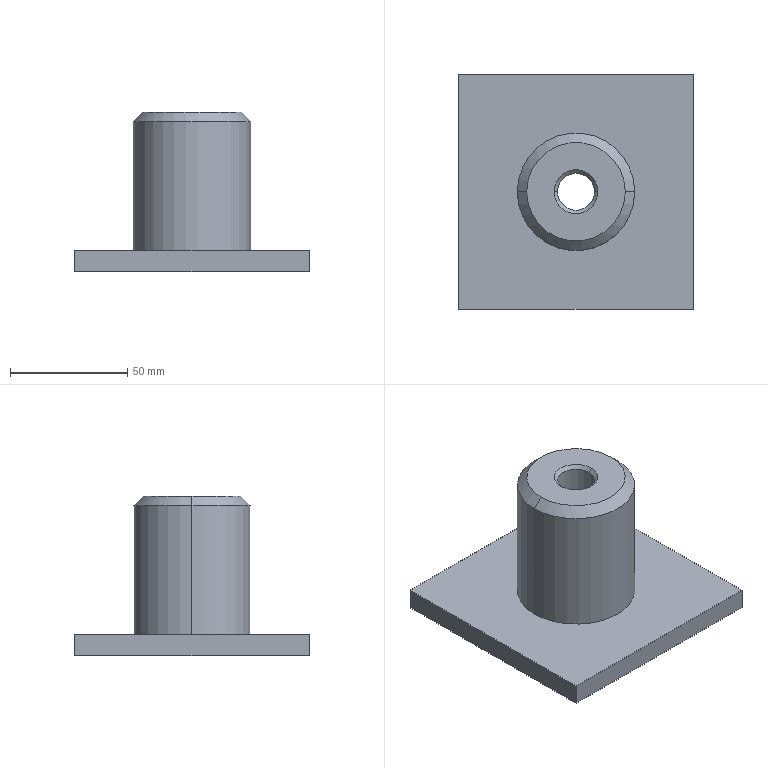Part | SolidWorks | features Chamfer 1, Extrusion 1, HoleWzd 1, ICE 1 | 1 solid | 17 faces | box 100 x 100 x 68 mm | volume 174571 mm3 | plane 7 | cone 6 | cylinder 4 | commonest cylinder face diameters 24 x2 50 x2
STEP:
#1=CARTESIAN_POINT('',(21.,0.,68.));
#2=VERTEX_POINT('',#1);
#3=CARTESIAN_POINT('',(-21.,0.,68.));
#4=VERTEX_POINT('',#3);
#5=CARTESIAN_POINT('',(0.,0.,68.));
#6=DIRECTION('',(0.,0.,1.));
#7=DIRECTION('',(1.,0.,0.));
#8=AXIS2_PLACEMENT_3D('',#5,#6,#7);
#9=CIRCLE('',#8,21.);
#10=EDGE_CURVE('',#2,#4,#9,.T.);
#11=ORIENTED_EDGE('',*,*,#10,.F.);
#12=CARTESIAN_POINT('',(25.,0.,64.));
#13=VERTEX_POINT('',#12);
#14=CARTESIAN_POINT('',(21.,0.,68.));
#15=DIRECTION('',(0.7071,0.,-0.7071));
#16=VECTOR('',#15,1000.);
#17=LINE('',#14,#16);
#18=EDGE_CURVE('',#2,#13,#17,.T.);
#19=ORIENTED_EDGE('',*,*,#18,.T.);
#20=CARTESIAN_POINT('',(-25.,0.,64.));
#21=VERTEX_POINT('',#20);
#22=CARTESIAN_POINT('',(0.,0.,64.));
#23=DIRECTION('',(0.,0.,-1.));
#24=DIRECTION('',(1.,0.,0.));
#25=AXIS2_PLACEMENT_3D('',#22,#23,#24);
#26=CIRCLE('',#25,25.);
#27=EDGE_CURVE('',#21,#13,#26,.T.);
#28=ORIENTED_EDGE('',*,*,#27,.F.);
#29=CARTESIAN_POINT('',(-21.,0.,68.));
#30=DIRECTION('',(-0.7071,0.,-0.7071));
#31=VECTOR('',#30,1000.);
#32=LINE('',#29,#31);
#33=EDGE_CURVE('',#4,#21,#32,.T.);
#34=ORIENTED_EDGE('',*,*,#33,.F.);
#35=EDGE_LOOP('',(#11,#19,#28,#34));
#36=FACE_OUTER_BOUND('',#35,.T.);
#37=CARTESIAN_POINT('',(0.,0.,68.));
#38=DIRECTION('',(0.,0.,-1.));
#39=DIRECTION('',(-1.,0.,0.));
#40=AXIS2_PLACEMENT_3D('',#37,#38,#39);
#41=CONICAL_SURFACE('',#40,21.,0.7854);
#42=ADVANCED_FACE('',(#36),#41,.T.);
#43=CARTESIAN_POINT('',(-7.842,0.,66.499));
#44=VERTEX_POINT('',#43);
#45=CARTESIAN_POINT('',(7.842,0.,66.499));
#46=VERTEX_POINT('',#45);
#47=CARTESIAN_POINT('',(0.,0.,66.499));
#48=DIRECTION('',(0.,0.,1.));
#49=DIRECTION('',(-1.,0.,0.));
#50=AXIS2_PLACEMENT_3D('',#47,#48,#49);
#51=CIRCLE('',#50,7.842);
#52=EDGE_CURVE('',#44,#46,#51,.T.);
#53=ORIENTED_EDGE('',*,*,#52,.F.);
#54=CARTESIAN_POINT('',(-9.343,0.,68.));
#55=VERTEX_POINT('',#54);
#56=CARTESIAN_POINT('',(-7.842,0.,66.499));
#57=DIRECTION('',(-0.7071,0.,0.7071));
#58=VECTOR('',#57,1000.);
#59=LINE('',#56,#58);
#60=EDGE_CURVE('',#44,#55,#59,.T.);
#61=ORIENTED_EDGE('',*,*,#60,.T.);
#62=CARTESIAN_POINT('',(9.343,0.,68.));
#63=VERTEX_POINT('',#62);
#64=CARTESIAN_POINT('',(0.,0.,68.));
#65=DIRECTION('',(0.,0.,-1.));
#66=DIRECTION('',(1.,0.,0.));
#67=AXIS2_PLACEMENT_3D('',#64,#65,#66);
#68=CIRCLE('',#67,9.343);
#69=EDGE_CURVE('',#63,#55,#68,.T.);
#70=ORIENTED_EDGE('',*,*,#69,.F.);
#71=CARTESIAN_POINT('',(7.842,0.,66.499));
#72=DIRECTION('',(0.7071,0.,0.7071));
#73=VECTOR('',#72,1000.);
#74=LINE('',#71,#73);
#75=EDGE_CURVE('',#46,#63,#74,.T.);
#76=ORIENTED_EDGE('',*,*,#75,.F.);
#77=EDGE_LOOP('',(#53,#61,#70,#76));
#78=FACE_OUTER_BOUND('',#77,.T.);
#79=CARTESIAN_POINT('',(0.,0.,66.499));
#80=DIRECTION('',(0.,0.,1.));
#81=DIRECTION('',(1.,0.,0.));
#82=AXIS2_PLACEMENT_3D('',#79,#80,#81);
#83=CONICAL_SURFACE('',#82,7.842,0.7854);
#84=ADVANCED_FACE('',(#78),#83,.F.);
#85=CARTESIAN_POINT('',(12.,0.,64.));
#86=VERTEX_POINT('',#85);
#87=CARTESIAN_POINT('',(-12.,0.,64.));
#88=VERTEX_POINT('',#87);
#89=CARTESIAN_POINT('',(0.,0.,64.));
#90=DIRECTION('',(0.,0.,-1.));
#91=DIRECTION('',(-1.,0.,0.));
#92=AXIS2_PLACEMENT_3D('',#89,#90,#91);
#93=CIRCLE('',#92,12.);
#94=EDGE_CURVE('',#86,#88,#93,.T.);
#95=ORIENTED_EDGE('',*,*,#94,.F.);
#96=CARTESIAN_POINT('',(12.,0.,0.));
#97=VERTEX_POINT('',#96);
#98=CARTESIAN_POINT('',(12.,0.,0.));
#99=DIRECTION('',(0.,0.,-1.));
#100=VECTOR('',#99,1000.);
#101=LINE('',#98,#100);
#102=EDGE_CURVE('',#86,#97,#101,.T.);
#103=ORIENTED_EDGE('',*,*,#102,.T.);
#104=CARTESIAN_POINT('',(-12.,0.,0.));
#105=VERTEX_POINT('',#104);
#106=CARTESIAN_POINT('',(0.,0.,0.));
#107=DIRECTION('',(0.,0.,-1.));
#108=DIRECTION('',(-1.,0.,0.));
#109=AXIS2_PLACEMENT_3D('',#106,#107,#108);
#110=CIRCLE('',#109,12.);
#111=EDGE_CURVE('',#97,#105,#110,.T.);
#112=ORIENTED_EDGE('',*,*,#111,.T.);
#113=CARTESIAN_POINT('',(-12.,0.,0.));
#114=DIRECTION('',(0.,0.,-1.));
#115=VECTOR('',#114,1000.);
#116=LINE('',#113,#115);
#117=EDGE_CURVE('',#88,#105,#116,.T.);
#118=ORIENTED_EDGE('',*,*,#117,.F.);
#119=EDGE_LOOP('',(#95,#103,#112,#118));
#120=FACE_OUTER_BOUND('',#119,.T.);
#121=CARTESIAN_POINT('',(0.,0.,0.));
#122=DIRECTION('',(0.,0.,-1.));
#123=DIRECTION('',(-1.,0.,0.));
#124=AXIS2_PLACEMENT_3D('',#121,#122,#123);
#125=CYLINDRICAL_SURFACE('',#124,12.);
#126=ADVANCED_FACE('',(#120),#125,.F.);
#127=ORIENTED_EDGE('',*,*,#52,.T.);
#128=CARTESIAN_POINT('',(12.,0.,64.));
#129=DIRECTION('',(0.8572,0.,-0.515));
#130=VECTOR('',#129,1000.);
#131=LINE('',#128,#130);
#132=EDGE_CURVE('',#46,#86,#131,.T.);
#133=ORIENTED_EDGE('',*,*,#132,.T.);
#134=ORIENTED_EDGE('',*,*,#94,.T.);
#135=CARTESIAN_POINT('',(-12.,0.,64.));
#136=DIRECTION('',(-0.8572,0.,-0.515));
#137=VECTOR('',#136,1000.);
#138=LINE('',#135,#137);
#139=EDGE_CURVE('',#44,#88,#138,.T.);
#140=ORIENTED_EDGE('',*,*,#139,.F.);
#141=EDGE_LOOP('',(#127,#133,#134,#140));
#142=FACE_OUTER_BOUND('',#141,.T.);
#143=CARTESIAN_POINT('',(0.,0.,64.));
#144=DIRECTION('',(0.,0.,-1.));
#145=DIRECTION('',(-1.,0.,0.));
#146=AXIS2_PLACEMENT_3D('',#143,#144,#145);
#147=CONICAL_SURFACE('',#146,12.,1.03);
#148=ADVANCED_FACE('',(#142),#147,.F.);
#149=ORIENTED_EDGE('',*,*,#27,.T.);
#150=CARTESIAN_POINT('',(25.,0.,9.));
#151=VERTEX_POINT('',#150);
#152=CARTESIAN_POINT('',(25.,0.,68.));
#153=DIRECTION('',(0.,0.,-1.));
#154=VECTOR('',#153,1000.);
#155=LINE('',#152,#154);
#156=EDGE_CURVE('',#13,#151,#155,.T.);
#157=ORIENTED_EDGE('',*,*,#156,.T.);
#158=CARTESIAN_POINT('',(-25.,0.,9.));
#159=VERTEX_POINT('',#158);
#160=CARTESIAN_POINT('',(0.,0.,9.));
#161=DIRECTION('',(0.,0.,1.));
#162=DIRECTION('',(1.,0.,0.));
#163=AXIS2_PLACEMENT_3D('',#160,#161,#162);
#164=CIRCLE('',#163,25.);
#165=EDGE_CURVE('',#151,#159,#164,.T.);
#166=ORIENTED_EDGE('',*,*,#165,.T.);
#167=CARTESIAN_POINT('',(-25.,0.,68.));
#168=DIRECTION('',(0.,0.,-1.));
#169=VECTOR('',#168,1000.);
#170=LINE('',#167,#169);
#171=EDGE_CURVE('',#21,#159,#170,.T.);
#172=ORIENTED_EDGE('',*,*,#171,.F.);
#173=EDGE_LOOP('',(#149,#157,#166,#172));
#174=FACE_OUTER_BOUND('',#173,.T.);
#175=CARTESIAN_POINT('',(0.,0.,68.));
#176=DIRECTION('',(0.,0.,-1.));
#177=DIRECTION('',(-1.,0.,0.));
#178=AXIS2_PLACEMENT_3D('',#175,#176,#177);
#179=CYLINDRICAL_SURFACE('',#178,25.);
#180=ADVANCED_FACE('',(#174),#179,.T.);
#181=CARTESIAN_POINT('',(-50.,50.,0.));
#182=VERTEX_POINT('',#181);
#183=CARTESIAN_POINT('',(-50.,-50.,0.));
#184=VERTEX_POINT('',#183);
#185=CARTESIAN_POINT('',(-50.,50.,0.));
#186=DIRECTION('',(0.,-1.,0.));
#187=VECTOR('',#186,1000.);
#188=LINE('',#185,#187);
#189=EDGE_CURVE('',#182,#184,#188,.T.);
#190=ORIENTED_EDGE('',*,*,#189,.T.);
#191=CARTESIAN_POINT('',(-50.,-50.,9.));
#192=VERTEX_POINT('',#191);
#193=CARTESIAN_POINT('',(-50.,-50.,9.));
#194=DIRECTION('',(0.,0.,-1.));
#195=VECTOR('',#194,1000.);
#196=LINE('',#193,#195);
#197=EDGE_CURVE('',#192,#184,#196,.T.);
#198=ORIENTED_EDGE('',*,*,#197,.F.);
#199=CARTESIAN_POINT('',(-50.,50.,9.));
#200=VERTEX_POINT('',#199);
#201=CARTESIAN_POINT('',(-50.,50.,9.));
#202=DIRECTION('',(0.,-1.,0.));
#203=VECTOR('',#202,1000.);
#204=LINE('',#201,#203);
#205=EDGE_CURVE('',#200,#192,#204,.T.);
#206=ORIENTED_EDGE('',*,*,#205,.F.);
#207=CARTESIAN_POINT('',(-50.,50.,9.));
#208=DIRECTION('',(0.,0.,-1.));
#209=VECTOR('',#208,1000.);
#210=LINE('',#207,#209);
#211=EDGE_CURVE('',#200,#182,#210,.T.);
#212=ORIENTED_EDGE('',*,*,#211,.T.);
#213=EDGE_LOOP('',(#190,#198,#206,#212));
#214=FACE_OUTER_BOUND('',#213,.T.);
#215=CARTESIAN_POINT('',(-50.,50.,9.));
#216=DIRECTION('',(1.,0.,0.));
#217=DIRECTION('',(0.,1.,0.));
#218=AXIS2_PLACEMENT_3D('',#215,#216,#217);
#219=PLANE('',#218);
#220=ADVANCED_FACE('',(#214),#219,.F.);
#221=CARTESIAN_POINT('',(50.,-50.,0.));
#222=VERTEX_POINT('',#221);
#223=CARTESIAN_POINT('',(50.,-50.,0.));
#224=DIRECTION('',(1.,0.,0.));
#225=VECTOR('',#224,1000.);
#226=LINE('',#223,#225);
#227=EDGE_CURVE('',#184,#222,#226,.T.);
#228=ORIENTED_EDGE('',*,*,#227,.T.);
#229=CARTESIAN_POINT('',(50.,-50.,9.));
#230=VERTEX_POINT('',#229);
#231=CARTESIAN_POINT('',(50.,-50.,9.));
#232=DIRECTION('',(0.,0.,-1.));
#233=VECTOR('',#232,1000.);
#234=LINE('',#231,#233);
#235=EDGE_CURVE('',#230,#222,#234,.T.);
#236=ORIENTED_EDGE('',*,*,#235,.F.);
#237=CARTESIAN_POINT('',(50.,-50.,9.));
#238=DIRECTION('',(1.,0.,0.));
#239=VECTOR('',#238,1000.);
#240=LINE('',#237,#239);
#241=EDGE_CURVE('',#192,#230,#240,.T.);
#242=ORIENTED_EDGE('',*,*,#241,.F.);
#243=ORIENTED_EDGE('',*,*,#197,.T.);
#244=EDGE_LOOP('',(#228,#236,#242,#243));
#245=FACE_OUTER_BOUND('',#244,.T.);
#246=CARTESIAN_POINT('',(50.,-50.,9.));
#247=DIRECTION('',(0.,1.,0.));
#248=DIRECTION('',(-1.,0.,0.));
#249=AXIS2_PLACEMENT_3D('',#246,#247,#248);
#250=PLANE('',#249);
#251=ADVANCED_FACE('',(#245),#250,.F.);
#252=CARTESIAN_POINT('',(50.,50.,0.));
#253=VERTEX_POINT('',#252);
#254=CARTESIAN_POINT('',(50.,50.,0.));
#255=DIRECTION('',(0.,1.,0.));
#256=VECTOR('',#255,1000.);
#257=LINE('',#254,#256);
#258=EDGE_CURVE('',#222,#253,#257,.T.);
#259=ORIENTED_EDGE('',*,*,#258,.T.);
#260=CARTESIAN_POINT('',(50.,50.,9.));
#261=VERTEX_POINT('',#260);
#262=CARTESIAN_POINT('',(50.,50.,9.));
#263=DIRECTION('',(0.,0.,-1.));
#264=VECTOR('',#263,1000.);
#265=LINE('',#262,#264);
#266=EDGE_CURVE('',#261,#253,#265,.T.);
#267=ORIENTED_EDGE('',*,*,#266,.F.);
#268=CARTESIAN_POINT('',(50.,50.,9.));
#269=DIRECTION('',(0.,1.,0.));
#270=VECTOR('',#269,1000.);
#271=LINE('',#268,#270);
#272=EDGE_CURVE('',#230,#261,#271,.T.);
#273=ORIENTED_EDGE('',*,*,#272,.F.);
#274=ORIENTED_EDGE('',*,*,#235,.T.);
#275=EDGE_LOOP('',(#259,#267,#273,#274));
#276=FACE_OUTER_BOUND('',#275,.T.);
#277=CARTESIAN_POINT('',(50.,50.,9.));
#278=DIRECTION('',(-1.,0.,0.));
#279=DIRECTION('',(0.,-1.,0.));
#280=AXIS2_PLACEMENT_3D('',#277,#278,#279);
#281=PLANE('',#280);
#282=ADVANCED_FACE('',(#276),#281,.F.);
#283=CARTESIAN_POINT('',(50.,50.,0.));
#284=DIRECTION('',(-1.,0.,0.));
#285=VECTOR('',#284,1000.);
#286=LINE('',#283,#285);
#287=EDGE_CURVE('',#253,#182,#286,.T.);
#288=ORIENTED_EDGE('',*,*,#287,.T.);
#289=ORIENTED_EDGE('',*,*,#211,.F.);
#290=CARTESIAN_POINT('',(50.,50.,9.));
#291=DIRECTION('',(-1.,0.,0.));
#292=VECTOR('',#291,1000.);
#293=LINE('',#290,#292);
#294=EDGE_CURVE('',#261,#200,#293,.T.);
#295=ORIENTED_EDGE('',*,*,#294,.F.);
#296=ORIENTED_EDGE('',*,*,#266,.T.);
#297=EDGE_LOOP('',(#288,#289,#295,#296));
#298=FACE_OUTER_BOUND('',#297,.T.);
#299=CARTESIAN_POINT('',(50.,50.,9.));
#300=DIRECTION('',(0.,-1.,0.));
#301=DIRECTION('',(1.,0.,0.));
#302=AXIS2_PLACEMENT_3D('',#299,#300,#301);
#303=PLANE('',#302);
#304=ADVANCED_FACE('',(#298),#303,.F.);
#305=CARTESIAN_POINT('',(0.,0.,9.));
#306=DIRECTION('',(0.,0.,1.));
#307=DIRECTION('',(1.,0.,0.));
#308=AXIS2_PLACEMENT_3D('',#305,#306,#307);
#309=CIRCLE('',#308,25.);
#310=EDGE_CURVE('',#159,#151,#309,.T.);
#311=ORIENTED_EDGE('',*,*,#310,.F.);
#312=ORIENTED_EDGE('',*,*,#165,.F.);
#313=EDGE_LOOP('',(#311,#312));
#314=FACE_BOUND('',#313,.T.);
#315=ORIENTED_EDGE('',*,*,#205,.T.);
#316=ORIENTED_EDGE('',*,*,#241,.T.);
#317=ORIENTED_EDGE('',*,*,#272,.T.);
#318=ORIENTED_EDGE('',*,*,#294,.T.);
#319=EDGE_LOOP('',(#315,#316,#317,#318));
#320=FACE_OUTER_BOUND('',#319,.T.);
#321=CARTESIAN_POINT('',(0.,0.,9.));
#322=DIRECTION('',(0.,0.,-1.));
#323=DIRECTION('',(-1.,0.,0.));
#324=AXIS2_PLACEMENT_3D('',#321,#322,#323);
#325=PLANE('',#324);
#326=ADVANCED_FACE('',(#314,#320),#325,.F.);
#327=CARTESIAN_POINT('',(0.,0.,0.));
#328=DIRECTION('',(0.,0.,-1.));
#329=DIRECTION('',(-1.,0.,0.));
#330=AXIS2_PLACEMENT_3D('',#327,#328,#329);
#331=CIRCLE('',#330,12.);
#332=EDGE_CURVE('',#105,#97,#331,.T.);
#333=ORIENTED_EDGE('',*,*,#332,.F.);
#334=ORIENTED_EDGE('',*,*,#111,.F.);
#335=EDGE_LOOP('',(#333,#334));
#336=FACE_BOUND('',#335,.T.);
#337=ORIENTED_EDGE('',*,*,#189,.F.);
#338=ORIENTED_EDGE('',*,*,#287,.F.);
#339=ORIENTED_EDGE('',*,*,#258,.F.);
#340=ORIENTED_EDGE('',*,*,#227,.F.);
#341=EDGE_LOOP('',(#337,#338,#339,#340));
#342=FACE_OUTER_BOUND('',#341,.T.);
#343=CARTESIAN_POINT('',(0.,0.,0.));
#344=DIRECTION('',(0.,0.,-1.));
#345=DIRECTION('',(-1.,0.,0.));
#346=AXIS2_PLACEMENT_3D('',#343,#344,#345);
#347=PLANE('',#346);
#348=ADVANCED_FACE('',(#336,#342),#347,.T.);
#349=ORIENTED_EDGE('',*,*,#156,.F.);
#350=CARTESIAN_POINT('',(0.,0.,64.));
#351=DIRECTION('',(0.,0.,-1.));
#352=DIRECTION('',(1.,0.,0.));
#353=AXIS2_PLACEMENT_3D('',#350,#351,#352);
#354=CIRCLE('',#353,25.);
#355=EDGE_CURVE('',#13,#21,#354,.T.);
#356=ORIENTED_EDGE('',*,*,#355,.T.);
#357=ORIENTED_EDGE('',*,*,#171,.T.);
#358=ORIENTED_EDGE('',*,*,#310,.T.);
#359=EDGE_LOOP('',(#349,#356,#357,#358));
#360=FACE_OUTER_BOUND('',#359,.T.);
#361=CARTESIAN_POINT('',(0.,0.,68.));
#362=DIRECTION('',(0.,0.,-1.));
#363=DIRECTION('',(-1.,0.,0.));
#364=AXIS2_PLACEMENT_3D('',#361,#362,#363);
#365=CYLINDRICAL_SURFACE('',#364,25.);
#366=ADVANCED_FACE('',(#360),#365,.T.);
#367=ORIENTED_EDGE('',*,*,#69,.T.);
#368=CARTESIAN_POINT('',(0.,0.,68.));
#369=DIRECTION('',(0.,0.,-1.));
#370=DIRECTION('',(1.,0.,0.));
#371=AXIS2_PLACEMENT_3D('',#368,#369,#370);
#372=CIRCLE('',#371,9.343);
#373=EDGE_CURVE('',#55,#63,#372,.T.);
#374=ORIENTED_EDGE('',*,*,#373,.T.);
#375=EDGE_LOOP('',(#367,#374));
#376=FACE_BOUND('',#375,.T.);
#377=CARTESIAN_POINT('',(0.,0.,68.));
#378=DIRECTION('',(0.,0.,1.));
#379=DIRECTION('',(1.,0.,0.));
#380=AXIS2_PLACEMENT_3D('',#377,#378,#379);
#381=CIRCLE('',#380,21.);
#382=EDGE_CURVE('',#4,#2,#381,.T.);
#383=ORIENTED_EDGE('',*,*,#382,.T.);
#384=ORIENTED_EDGE('',*,*,#10,.T.);
#385=EDGE_LOOP('',(#383,#384));
#386=FACE_OUTER_BOUND('',#385,.T.);
#387=CARTESIAN_POINT('',(0.,0.,68.));
#388=DIRECTION('',(0.,0.,1.));
#389=DIRECTION('',(1.,0.,0.));
#390=AXIS2_PLACEMENT_3D('',#387,#388,#389);
#391=PLANE('',#390);
#392=ADVANCED_FACE('',(#376,#386),#391,.T.);
#393=ORIENTED_EDGE('',*,*,#132,.F.);
#394=CARTESIAN_POINT('',(0.,0.,66.499));
#395=DIRECTION('',(0.,0.,1.));
#396=DIRECTION('',(-1.,0.,0.));
#397=AXIS2_PLACEMENT_3D('',#394,#395,#396);
#398=CIRCLE('',#397,7.842);
#399=EDGE_CURVE('',#46,#44,#398,.T.);
#400=ORIENTED_EDGE('',*,*,#399,.T.);
#401=ORIENTED_EDGE('',*,*,#139,.T.);
#402=CARTESIAN_POINT('',(0.,0.,64.));
#403=DIRECTION('',(0.,0.,-1.));
#404=DIRECTION('',(-1.,0.,0.));
#405=AXIS2_PLACEMENT_3D('',#402,#403,#404);
#406=CIRCLE('',#405,12.);
#407=EDGE_CURVE('',#88,#86,#406,.T.);
#408=ORIENTED_EDGE('',*,*,#407,.T.);
#409=EDGE_LOOP('',(#393,#400,#401,#408));
#410=FACE_OUTER_BOUND('',#409,.T.);
#411=CARTESIAN_POINT('',(0.,0.,64.));
#412=DIRECTION('',(0.,0.,-1.));
#413=DIRECTION('',(-1.,0.,0.));
#414=AXIS2_PLACEMENT_3D('',#411,#412,#413);
#415=CONICAL_SURFACE('',#414,12.,1.03);
#416=ADVANCED_FACE('',(#410),#415,.F.);
#417=ORIENTED_EDGE('',*,*,#102,.F.);
#418=ORIENTED_EDGE('',*,*,#407,.F.);
#419=ORIENTED_EDGE('',*,*,#117,.T.);
#420=ORIENTED_EDGE('',*,*,#332,.T.);
#421=EDGE_LOOP('',(#417,#418,#419,#420));
#422=FACE_OUTER_BOUND('',#421,.T.);
#423=CARTESIAN_POINT('',(0.,0.,0.));
#424=DIRECTION('',(0.,0.,-1.));
#425=DIRECTION('',(-1.,0.,0.));
#426=AXIS2_PLACEMENT_3D('',#423,#424,#425);
#427=CYLINDRICAL_SURFACE('',#426,12.);
#428=ADVANCED_FACE('',(#422),#427,.F.);
#429=ORIENTED_EDGE('',*,*,#60,.F.);
#430=ORIENTED_EDGE('',*,*,#399,.F.);
#431=ORIENTED_EDGE('',*,*,#75,.T.);
#432=ORIENTED_EDGE('',*,*,#373,.F.);
#433=EDGE_LOOP('',(#429,#430,#431,#432));
#434=FACE_OUTER_BOUND('',#433,.T.);
#435=CARTESIAN_POINT('',(0.,0.,66.499));
#436=DIRECTION('',(0.,0.,1.));
#437=DIRECTION('',(1.,0.,0.));
#438=AXIS2_PLACEMENT_3D('',#435,#436,#437);
#439=CONICAL_SURFACE('',#438,7.842,0.7854);
#440=ADVANCED_FACE('',(#434),#439,.F.);
#441=ORIENTED_EDGE('',*,*,#18,.F.);
#442=ORIENTED_EDGE('',*,*,#382,.F.);
#443=ORIENTED_EDGE('',*,*,#33,.T.);
#444=ORIENTED_EDGE('',*,*,#355,.F.);
#445=EDGE_LOOP('',(#441,#442,#443,#444));
#446=FACE_OUTER_BOUND('',#445,.T.);
#447=CARTESIAN_POINT('',(0.,0.,68.));
#448=DIRECTION('',(0.,0.,-1.));
#449=DIRECTION('',(-1.,0.,0.));
#450=AXIS2_PLACEMENT_3D('',#447,#448,#449);
#451=CONICAL_SURFACE('',#450,21.,0.7854);
#452=ADVANCED_FACE('',(#446),#451,.T.);
#453=CLOSED_SHELL('',(#42,#84,#126,#148,#180,#220,#251,#282,#304,#326,#348,#366,#392,#416,#428,#440,#452));
#454=MANIFOLD_SOLID_BREP('',#453);
#455=CARTESIAN_POINT('',(0.,0.,0.));
#456=DIRECTION('',(0.,0.,1.));
#457=DIRECTION('',(1.,0.,0.));
#458=AXIS2_PLACEMENT_3D('',#455,#456,#457);
#459=(LENGTH_UNIT()NAMED_UNIT(*)SI_UNIT(.MILLI.,.METRE.));
#460=UNCERTAINTY_MEASURE_WITH_UNIT(LENGTH_MEASURE(0.00001),#459,'','');
#461=(NAMED_UNIT(*)PLANE_ANGLE_UNIT()SI_UNIT($,.RADIAN.));
#462=(NAMED_UNIT(*)SI_UNIT($,.STERADIAN.)SOLID_ANGLE_UNIT());
#463=(GEOMETRIC_REPRESENTATION_CONTEXT(3)GLOBAL_UNCERTAINTY_ASSIGNED_CONTEXT((#460))GLOBAL_UNIT_ASSIGNED_CONTEXT((#459,#461,#462))REPRESENTATION_CONTEXT('',''));
#464=ADVANCED_BREP_SHAPE_REPRESENTATION('',(#454,#458),#463);